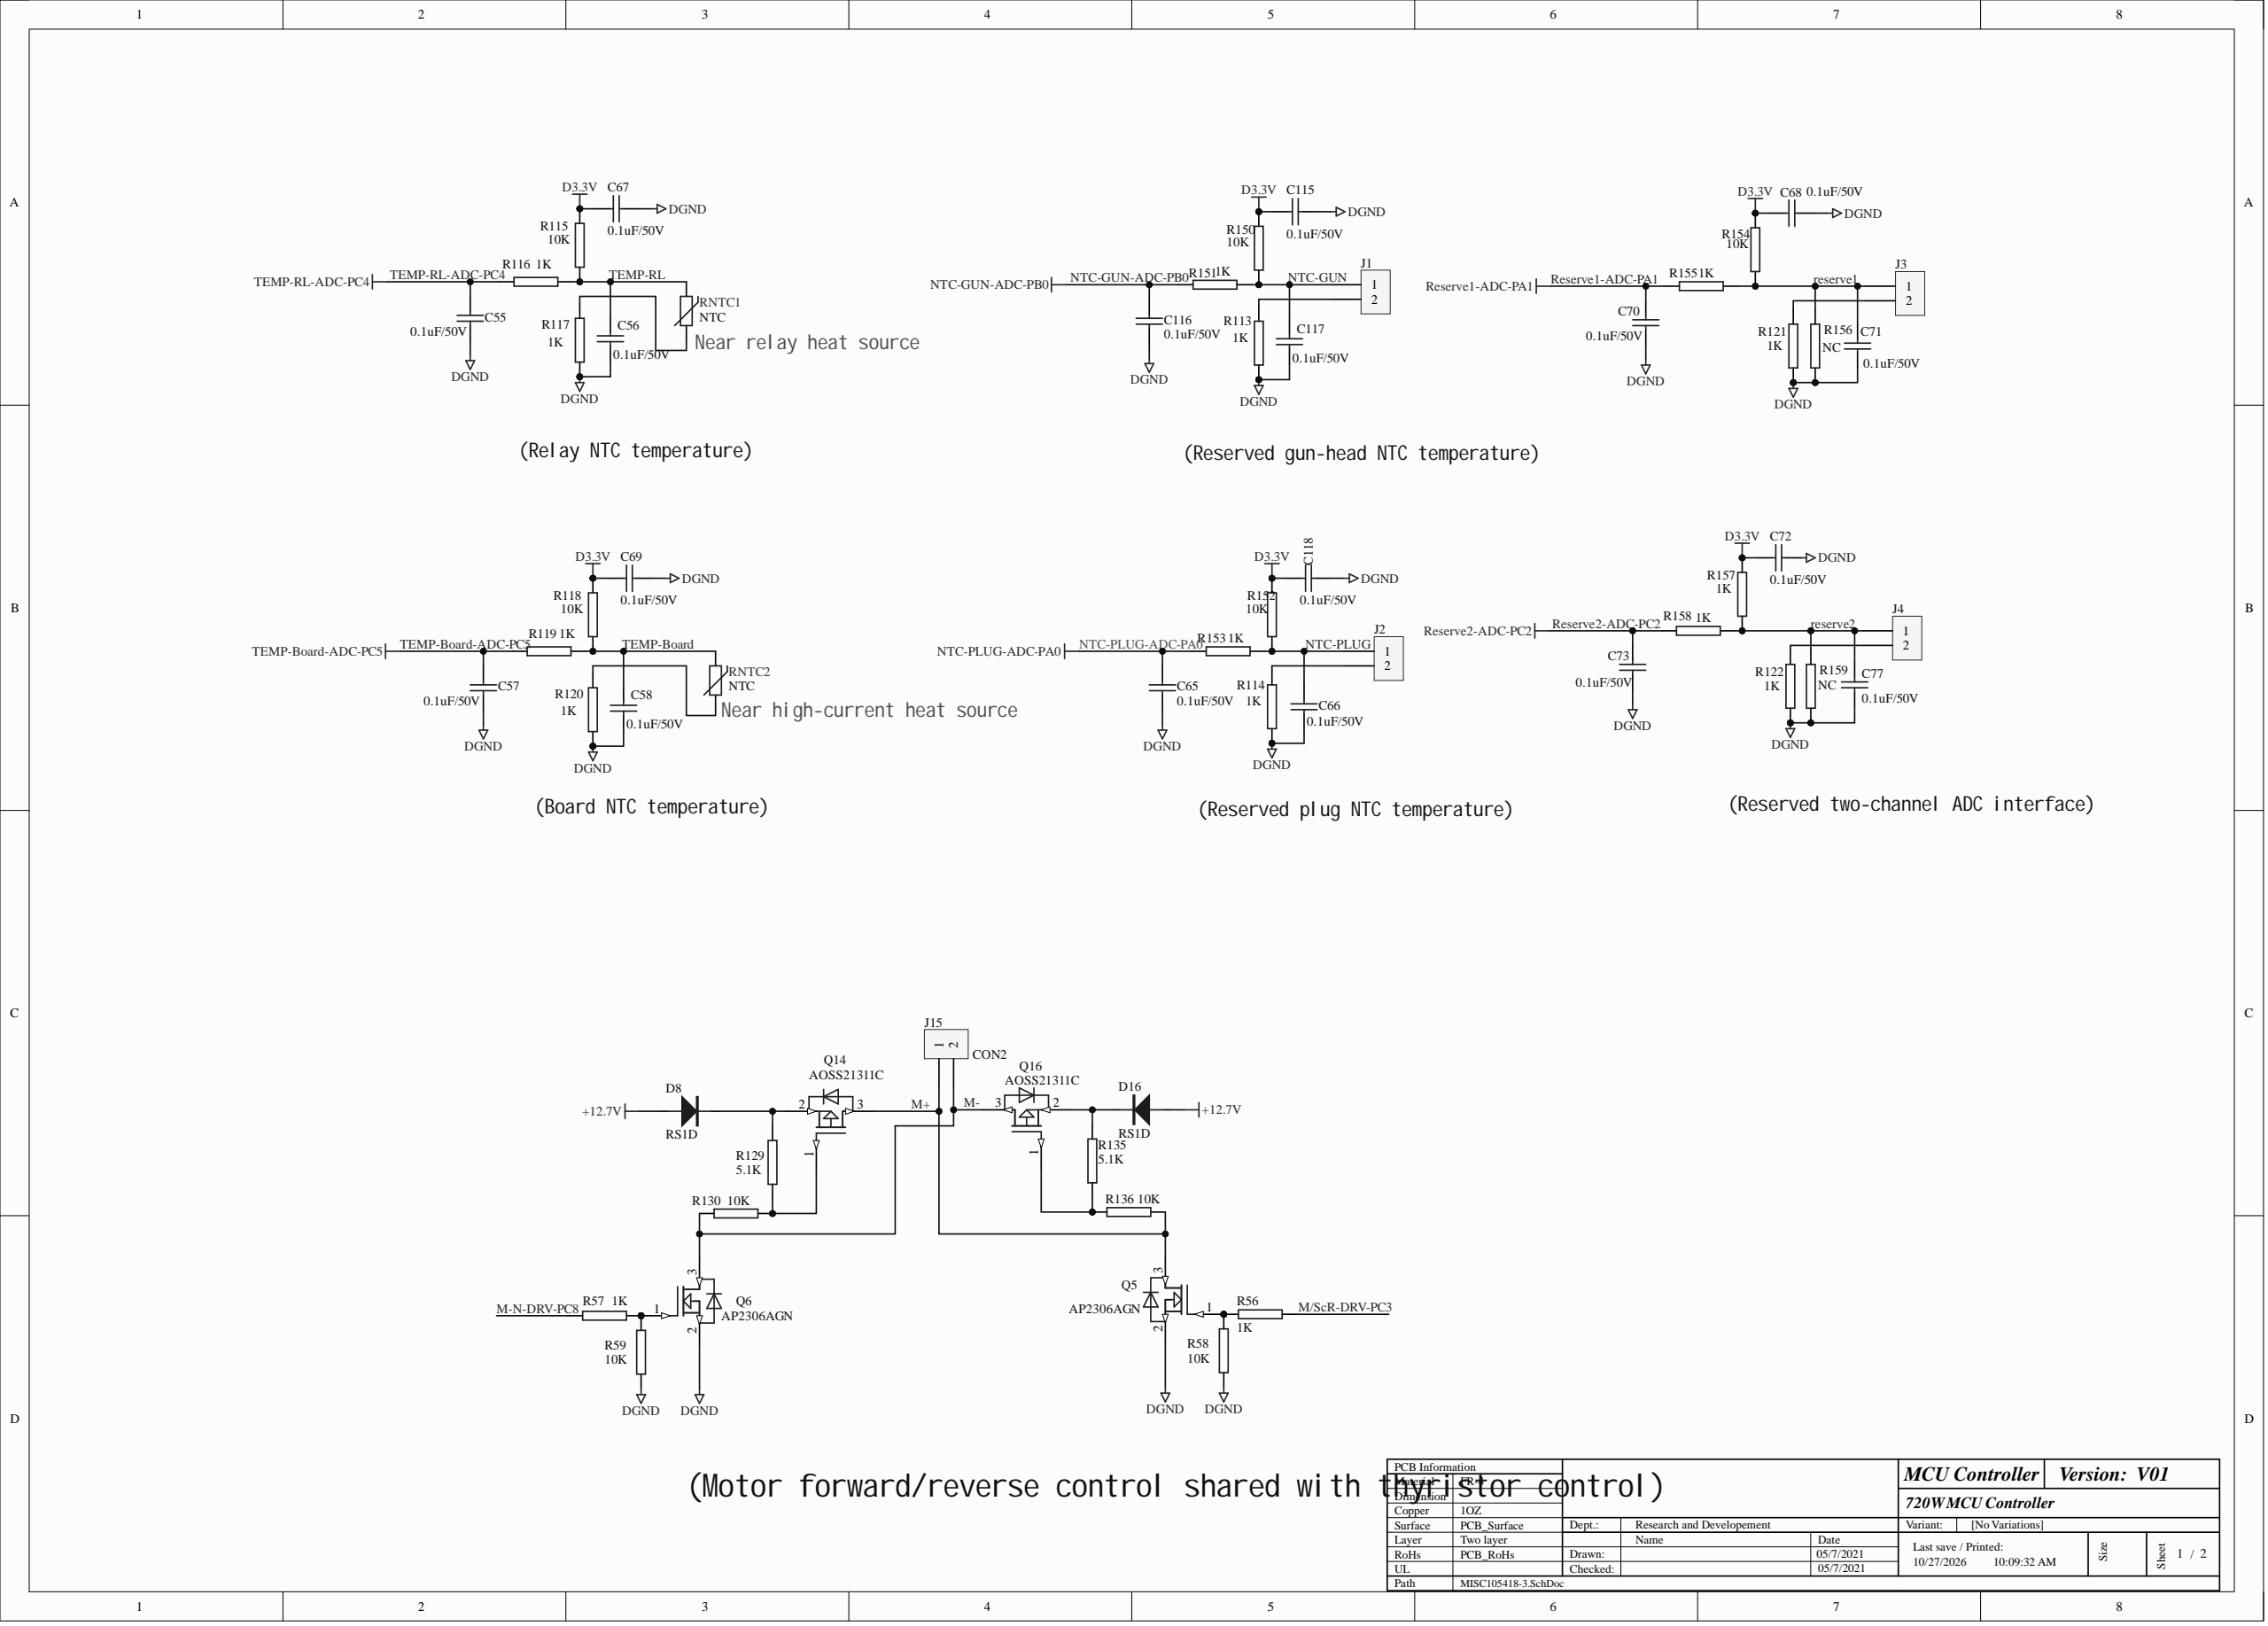Circuit board | Altium Designer | 455 parts | 280 nets | one sheet of the schematic
Parts on this sheet (reference | value | footprint):
C55 | 0.1uF/50V | C0603-T
C56 | 0.1uF/50V | C0603-T
C57 | 0.1uF/50V | C0603-T
C58 | 0.1uF/50V | C0603-T
C65 | 0.1uF/50V | C0603-T
C66 | 0.1uF/50V | C0603-T
C67 | 0.1uF/50V | C0603-T
C68 | 0.1uF/50V | C0603-T
C69 | 0.1uF/50V | C0603-T
C70 | 0.1uF/50V | C0603-T
C71 | 0.1uF/50V | C0603-T
C72 | 0.1uF/50V | C0603-T
C73 | 0.1uF/50V | C0603-T
C77 | 0.1uF/50V | C0603-T
C115 | 0.1uF/50V | C0603-T
C116 | 0.1uF/50V | C0603-T
C117 | 0.1uF/50V | C0603-T
C118 | 0.1uF/50V | C0603-T
D8 | RS1D | SMA
D16 | RS1D | SMA
J1 | CON2 | CON2-2.54
J2 | CON2 | CON2-2.54
J3 | CON2 | CON2-2.54
J4 | CON2 | CON2-2.54
J15 | CON2 | CON2-3.81
Q5 | AP2306AGN | SOT-23-T
Q6 | AP2306AGN | SOT-23-T
Q14 | AOSS21311C | SOT-23-T
Q16 | AOSS21311C | SOT-23-T
R56 | 1K | R0603-T
R57 | 1K | R0603-T
R58 | 10K | R0805-T
R59 | 10K | R0805-T
R113 | 1K | R0603-T
R114 | 1K | R0603-T
R115 | 10K | R0603-T
R116 | 1K | R0603-T
R117 | 1K | R0603-T
R118 | 10K | R0603-T
R119 | 1K | R0603-T
R120 | 1K | R0603-T
R121 | 1K | R0603-T
R122 | 1K | R0603-T
R129 | 5.1K | R0805-T
R130 | 10K | R0805-T
R135 | 5.1K | R0805-T
R136 | 10K | R0805-T
R150 | 10K | R0603-T
R152 | 10K | R0603-T
R153 | 1K | R0603-T
R154 | 10K | R0603-T
R156 | NC | R0603-T
R157 | 1K | R0603-T
R158 | 1K | R0603-T
R159 | NC | R0603-T
RNTC1 | NTC | R0603-t
RNTC2 | NTC | R0603-t
Nets of these parts (net: part-pin ...):
TEMP-RL-ADC-PC4: C55-1 R116-2
TEMP-RL: C56-2 R115-1 R116-1 RNTC1-2
TEMP-Board-ADC-PC5: C57-1 R119-2
TEMP-Board: C58-2 R118-1 R119-1 RNTC2-2
Reserve2-ADC-PC2: C73-1 R158-2
reserve2: C77-1 J4-1 R157-1 R158-1 R159-2
Reserve1-ADC-PA1: C70-1
reserve1: C71-1 J3-1 R154-1 R156-2
NTC-PLUG-ADC-PA0: C65-1 R153-2
NTC-PLUG: C66-1 J2-1 R152-1 R153-1
NTC-GUN-ADC-PB0: C116-1
NTC-GUN: C117-2 J1-1 R150-1
NetR120_2: R120-2 RNTC2-1
NetR117_2: R117-2 RNTC1-1
NetQ16_1: Q16-1 R135-2 R136-2
NetQ14_1: Q14-1 R129-2 R130-2
NetQ6_1: Q6-1 R57-1 R59-2
NetQ5_1: Q5-1 R56-2 R58-2
NetJ4_2: J4-2 R122-1
NetJ3_2: J3-2 R121-1
NetJ2_2: J2-2 R114-2
NetJ1_2: J1-2 R113-2
NetD16_2: D16-2 Q16-2 R135-1
NetD8_2: D8-2 Q14-2 R129-1
M/ScR-DRV-PC3: R56-1
M-N-DRV-PC8: R57-2
M-: J15-2 Q6-3 Q16-3 R130-1
M+: J15-1 Q5-3 Q14-3 R136-1
D3.3V: C67-2 C68-2 C69-2 C72-2 C115-2 C118-2 R115-2 R118-2 R150-2 R152-2 R154-2 R157-2
-: C55-2 C56-1 C57-2 C58-1 C65-2 C66-2 C67-1 C68-1 C69-1 C70-2 C71-2 C72-1 C73-2 C77-2 C115-1 C116-2 C117-1 C118-1 Q5-2 Q6-2 R58-1 R59-1 R113-1 R114-1 R117-1 R120-1 R121-2 R122-2 R156-1 R159-1
+12.7V: D8-1 D16-1